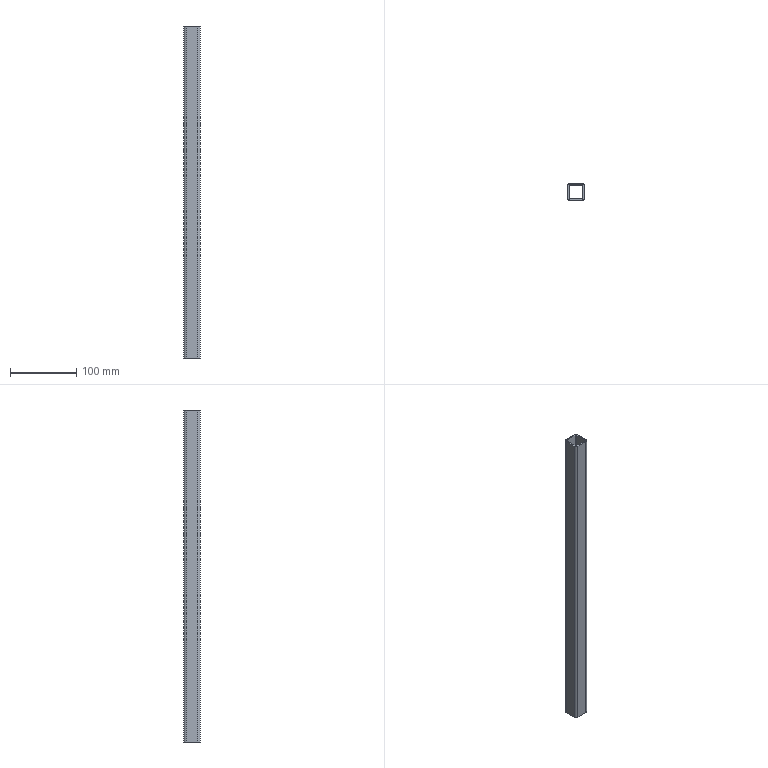Part | SolidWorks | features Extrusion 1 | 1 solid | 18 faces | box 25 x 25 x 500 mm | volume 86850 mm3 | plane 10 | cylinder 8 | commonest cylinder face diameters 4 x4 8 x4
STEP:
#1=CARTESIAN_POINT('',(0.,4.,500.));
#2=VERTEX_POINT('',#1);
#3=CARTESIAN_POINT('',(4.,0.,500.));
#4=VERTEX_POINT('',#3);
#5=CARTESIAN_POINT('',(4.,4.,500.));
#6=DIRECTION('',(0.,0.,1.));
#7=DIRECTION('',(-1.,0.,0.));
#8=AXIS2_PLACEMENT_3D('',#5,#6,#7);
#9=CIRCLE('',#8,4.);
#10=EDGE_CURVE('',#2,#4,#9,.T.);
#11=ORIENTED_EDGE('',*,*,#10,.T.);
#12=CARTESIAN_POINT('',(21.,0.,500.));
#13=VERTEX_POINT('',#12);
#14=CARTESIAN_POINT('',(4.,0.,500.));
#15=DIRECTION('',(1.,0.,0.));
#16=VECTOR('',#15,1000.);
#17=LINE('',#14,#16);
#18=EDGE_CURVE('',#4,#13,#17,.T.);
#19=ORIENTED_EDGE('',*,*,#18,.T.);
#20=CARTESIAN_POINT('',(25.,4.,500.));
#21=VERTEX_POINT('',#20);
#22=CARTESIAN_POINT('',(21.,4.,500.));
#23=DIRECTION('',(0.,0.,1.));
#24=DIRECTION('',(1.,0.,0.));
#25=AXIS2_PLACEMENT_3D('',#22,#23,#24);
#26=CIRCLE('',#25,4.);
#27=EDGE_CURVE('',#13,#21,#26,.T.);
#28=ORIENTED_EDGE('',*,*,#27,.T.);
#29=CARTESIAN_POINT('',(25.,21.,500.));
#30=VERTEX_POINT('',#29);
#31=CARTESIAN_POINT('',(25.,4.,500.));
#32=DIRECTION('',(0.,1.,0.));
#33=VECTOR('',#32,1000.);
#34=LINE('',#31,#33);
#35=EDGE_CURVE('',#21,#30,#34,.T.);
#36=ORIENTED_EDGE('',*,*,#35,.T.);
#37=CARTESIAN_POINT('',(21.,25.,500.));
#38=VERTEX_POINT('',#37);
#39=CARTESIAN_POINT('',(21.,21.,500.));
#40=DIRECTION('',(0.,0.,1.));
#41=DIRECTION('',(-1.,0.,0.));
#42=AXIS2_PLACEMENT_3D('',#39,#40,#41);
#43=CIRCLE('',#42,4.);
#44=EDGE_CURVE('',#30,#38,#43,.T.);
#45=ORIENTED_EDGE('',*,*,#44,.T.);
#46=CARTESIAN_POINT('',(4.,25.,500.));
#47=VERTEX_POINT('',#46);
#48=CARTESIAN_POINT('',(4.,25.,500.));
#49=DIRECTION('',(-1.,0.,0.));
#50=VECTOR('',#49,1000.);
#51=LINE('',#48,#50);
#52=EDGE_CURVE('',#38,#47,#51,.T.);
#53=ORIENTED_EDGE('',*,*,#52,.T.);
#54=CARTESIAN_POINT('',(0.,21.,500.));
#55=VERTEX_POINT('',#54);
#56=CARTESIAN_POINT('',(4.,21.,500.));
#57=DIRECTION('',(0.,0.,1.));
#58=DIRECTION('',(-1.,0.,0.));
#59=AXIS2_PLACEMENT_3D('',#56,#57,#58);
#60=CIRCLE('',#59,4.);
#61=EDGE_CURVE('',#47,#55,#60,.T.);
#62=ORIENTED_EDGE('',*,*,#61,.T.);
#63=CARTESIAN_POINT('',(0.,4.,500.));
#64=DIRECTION('',(0.,-1.,0.));
#65=VECTOR('',#64,1000.);
#66=LINE('',#63,#65);
#67=EDGE_CURVE('',#55,#2,#66,.T.);
#68=ORIENTED_EDGE('',*,*,#67,.T.);
#69=EDGE_LOOP('',(#11,#19,#28,#36,#45,#53,#62,#68));
#70=FACE_OUTER_BOUND('',#69,.T.);
#71=CARTESIAN_POINT('',(23.,21.,500.));
#72=VERTEX_POINT('',#71);
#73=CARTESIAN_POINT('',(21.,23.,500.));
#74=VERTEX_POINT('',#73);
#75=CARTESIAN_POINT('',(21.,21.,500.));
#76=DIRECTION('',(0.,0.,1.));
#77=DIRECTION('',(-1.,0.,0.));
#78=AXIS2_PLACEMENT_3D('',#75,#76,#77);
#79=CIRCLE('',#78,2.);
#80=EDGE_CURVE('',#72,#74,#79,.T.);
#81=ORIENTED_EDGE('',*,*,#80,.F.);
#82=CARTESIAN_POINT('',(23.,4.,500.));
#83=VERTEX_POINT('',#82);
#84=CARTESIAN_POINT('',(23.,4.,500.));
#85=DIRECTION('',(0.,1.,0.));
#86=VECTOR('',#85,1000.);
#87=LINE('',#84,#86);
#88=EDGE_CURVE('',#83,#72,#87,.T.);
#89=ORIENTED_EDGE('',*,*,#88,.F.);
#90=CARTESIAN_POINT('',(21.,2.,500.));
#91=VERTEX_POINT('',#90);
#92=CARTESIAN_POINT('',(21.,4.,500.));
#93=DIRECTION('',(0.,0.,1.));
#94=DIRECTION('',(1.,0.,0.));
#95=AXIS2_PLACEMENT_3D('',#92,#93,#94);
#96=CIRCLE('',#95,2.);
#97=EDGE_CURVE('',#91,#83,#96,.T.);
#98=ORIENTED_EDGE('',*,*,#97,.F.);
#99=CARTESIAN_POINT('',(4.,2.,500.));
#100=VERTEX_POINT('',#99);
#101=CARTESIAN_POINT('',(4.,2.,500.));
#102=DIRECTION('',(1.,0.,0.));
#103=VECTOR('',#102,1000.);
#104=LINE('',#101,#103);
#105=EDGE_CURVE('',#100,#91,#104,.T.);
#106=ORIENTED_EDGE('',*,*,#105,.F.);
#107=CARTESIAN_POINT('',(2.,4.,500.));
#108=VERTEX_POINT('',#107);
#109=CARTESIAN_POINT('',(4.,4.,500.));
#110=DIRECTION('',(0.,0.,1.));
#111=DIRECTION('',(-1.,0.,0.));
#112=AXIS2_PLACEMENT_3D('',#109,#110,#111);
#113=CIRCLE('',#112,2.);
#114=EDGE_CURVE('',#108,#100,#113,.T.);
#115=ORIENTED_EDGE('',*,*,#114,.F.);
#116=CARTESIAN_POINT('',(2.,21.,500.));
#117=VERTEX_POINT('',#116);
#118=CARTESIAN_POINT('',(2.,4.,500.));
#119=DIRECTION('',(0.,-1.,0.));
#120=VECTOR('',#119,1000.);
#121=LINE('',#118,#120);
#122=EDGE_CURVE('',#117,#108,#121,.T.);
#123=ORIENTED_EDGE('',*,*,#122,.F.);
#124=CARTESIAN_POINT('',(4.,23.,500.));
#125=VERTEX_POINT('',#124);
#126=CARTESIAN_POINT('',(4.,21.,500.));
#127=DIRECTION('',(0.,0.,1.));
#128=DIRECTION('',(-1.,0.,0.));
#129=AXIS2_PLACEMENT_3D('',#126,#127,#128);
#130=CIRCLE('',#129,2.);
#131=EDGE_CURVE('',#125,#117,#130,.T.);
#132=ORIENTED_EDGE('',*,*,#131,.F.);
#133=CARTESIAN_POINT('',(4.,23.,500.));
#134=DIRECTION('',(-1.,0.,0.));
#135=VECTOR('',#134,1000.);
#136=LINE('',#133,#135);
#137=EDGE_CURVE('',#74,#125,#136,.T.);
#138=ORIENTED_EDGE('',*,*,#137,.F.);
#139=EDGE_LOOP('',(#81,#89,#98,#106,#115,#123,#132,#138));
#140=FACE_BOUND('',#139,.T.);
#141=CARTESIAN_POINT('',(4.,4.,500.));
#142=DIRECTION('',(0.,0.,-1.));
#143=DIRECTION('',(-1.,0.,0.));
#144=AXIS2_PLACEMENT_3D('',#141,#142,#143);
#145=PLANE('',#144);
#146=ADVANCED_FACE('',(#70,#140),#145,.F.);
#147=CARTESIAN_POINT('',(0.,4.,0.));
#148=VERTEX_POINT('',#147);
#149=CARTESIAN_POINT('',(4.,0.,0.));
#150=VERTEX_POINT('',#149);
#151=CARTESIAN_POINT('',(4.,4.,0.));
#152=DIRECTION('',(0.,0.,1.));
#153=DIRECTION('',(-1.,0.,0.));
#154=AXIS2_PLACEMENT_3D('',#151,#152,#153);
#155=CIRCLE('',#154,4.);
#156=EDGE_CURVE('',#148,#150,#155,.T.);
#157=ORIENTED_EDGE('',*,*,#156,.F.);
#158=CARTESIAN_POINT('',(0.,21.,0.));
#159=VERTEX_POINT('',#158);
#160=CARTESIAN_POINT('',(0.,4.,0.));
#161=DIRECTION('',(0.,-1.,0.));
#162=VECTOR('',#161,1000.);
#163=LINE('',#160,#162);
#164=EDGE_CURVE('',#159,#148,#163,.T.);
#165=ORIENTED_EDGE('',*,*,#164,.F.);
#166=CARTESIAN_POINT('',(4.,25.,0.));
#167=VERTEX_POINT('',#166);
#168=CARTESIAN_POINT('',(4.,21.,0.));
#169=DIRECTION('',(0.,0.,1.));
#170=DIRECTION('',(-1.,0.,0.));
#171=AXIS2_PLACEMENT_3D('',#168,#169,#170);
#172=CIRCLE('',#171,4.);
#173=EDGE_CURVE('',#167,#159,#172,.T.);
#174=ORIENTED_EDGE('',*,*,#173,.F.);
#175=CARTESIAN_POINT('',(21.,25.,0.));
#176=VERTEX_POINT('',#175);
#177=CARTESIAN_POINT('',(4.,25.,0.));
#178=DIRECTION('',(-1.,0.,0.));
#179=VECTOR('',#178,1000.);
#180=LINE('',#177,#179);
#181=EDGE_CURVE('',#176,#167,#180,.T.);
#182=ORIENTED_EDGE('',*,*,#181,.F.);
#183=CARTESIAN_POINT('',(25.,21.,0.));
#184=VERTEX_POINT('',#183);
#185=CARTESIAN_POINT('',(21.,21.,0.));
#186=DIRECTION('',(0.,0.,1.));
#187=DIRECTION('',(-1.,0.,0.));
#188=AXIS2_PLACEMENT_3D('',#185,#186,#187);
#189=CIRCLE('',#188,4.);
#190=EDGE_CURVE('',#184,#176,#189,.T.);
#191=ORIENTED_EDGE('',*,*,#190,.F.);
#192=CARTESIAN_POINT('',(25.,4.,0.));
#193=VERTEX_POINT('',#192);
#194=CARTESIAN_POINT('',(25.,4.,0.));
#195=DIRECTION('',(0.,1.,0.));
#196=VECTOR('',#195,1000.);
#197=LINE('',#194,#196);
#198=EDGE_CURVE('',#193,#184,#197,.T.);
#199=ORIENTED_EDGE('',*,*,#198,.F.);
#200=CARTESIAN_POINT('',(21.,0.,0.));
#201=VERTEX_POINT('',#200);
#202=CARTESIAN_POINT('',(21.,4.,0.));
#203=DIRECTION('',(0.,0.,1.));
#204=DIRECTION('',(1.,0.,0.));
#205=AXIS2_PLACEMENT_3D('',#202,#203,#204);
#206=CIRCLE('',#205,4.);
#207=EDGE_CURVE('',#201,#193,#206,.T.);
#208=ORIENTED_EDGE('',*,*,#207,.F.);
#209=CARTESIAN_POINT('',(4.,0.,0.));
#210=DIRECTION('',(1.,0.,0.));
#211=VECTOR('',#210,1000.);
#212=LINE('',#209,#211);
#213=EDGE_CURVE('',#150,#201,#212,.T.);
#214=ORIENTED_EDGE('',*,*,#213,.F.);
#215=EDGE_LOOP('',(#157,#165,#174,#182,#191,#199,#208,#214));
#216=FACE_OUTER_BOUND('',#215,.T.);
#217=CARTESIAN_POINT('',(23.,4.,0.));
#218=VERTEX_POINT('',#217);
#219=CARTESIAN_POINT('',(23.,21.,0.));
#220=VERTEX_POINT('',#219);
#221=CARTESIAN_POINT('',(23.,4.,0.));
#222=DIRECTION('',(0.,1.,0.));
#223=VECTOR('',#222,1000.);
#224=LINE('',#221,#223);
#225=EDGE_CURVE('',#218,#220,#224,.T.);
#226=ORIENTED_EDGE('',*,*,#225,.T.);
#227=CARTESIAN_POINT('',(21.,23.,0.));
#228=VERTEX_POINT('',#227);
#229=CARTESIAN_POINT('',(21.,21.,0.));
#230=DIRECTION('',(0.,0.,1.));
#231=DIRECTION('',(-1.,0.,0.));
#232=AXIS2_PLACEMENT_3D('',#229,#230,#231);
#233=CIRCLE('',#232,2.);
#234=EDGE_CURVE('',#220,#228,#233,.T.);
#235=ORIENTED_EDGE('',*,*,#234,.T.);
#236=CARTESIAN_POINT('',(4.,23.,0.));
#237=VERTEX_POINT('',#236);
#238=CARTESIAN_POINT('',(4.,23.,0.));
#239=DIRECTION('',(-1.,0.,0.));
#240=VECTOR('',#239,1000.);
#241=LINE('',#238,#240);
#242=EDGE_CURVE('',#228,#237,#241,.T.);
#243=ORIENTED_EDGE('',*,*,#242,.T.);
#244=CARTESIAN_POINT('',(2.,21.,0.));
#245=VERTEX_POINT('',#244);
#246=CARTESIAN_POINT('',(4.,21.,0.));
#247=DIRECTION('',(0.,0.,1.));
#248=DIRECTION('',(-1.,0.,0.));
#249=AXIS2_PLACEMENT_3D('',#246,#247,#248);
#250=CIRCLE('',#249,2.);
#251=EDGE_CURVE('',#237,#245,#250,.T.);
#252=ORIENTED_EDGE('',*,*,#251,.T.);
#253=CARTESIAN_POINT('',(2.,4.,0.));
#254=VERTEX_POINT('',#253);
#255=CARTESIAN_POINT('',(2.,4.,0.));
#256=DIRECTION('',(0.,-1.,0.));
#257=VECTOR('',#256,1000.);
#258=LINE('',#255,#257);
#259=EDGE_CURVE('',#245,#254,#258,.T.);
#260=ORIENTED_EDGE('',*,*,#259,.T.);
#261=CARTESIAN_POINT('',(4.,2.,0.));
#262=VERTEX_POINT('',#261);
#263=CARTESIAN_POINT('',(4.,4.,0.));
#264=DIRECTION('',(0.,0.,1.));
#265=DIRECTION('',(-1.,0.,0.));
#266=AXIS2_PLACEMENT_3D('',#263,#264,#265);
#267=CIRCLE('',#266,2.);
#268=EDGE_CURVE('',#254,#262,#267,.T.);
#269=ORIENTED_EDGE('',*,*,#268,.T.);
#270=CARTESIAN_POINT('',(21.,2.,0.));
#271=VERTEX_POINT('',#270);
#272=CARTESIAN_POINT('',(4.,2.,0.));
#273=DIRECTION('',(1.,0.,0.));
#274=VECTOR('',#273,1000.);
#275=LINE('',#272,#274);
#276=EDGE_CURVE('',#262,#271,#275,.T.);
#277=ORIENTED_EDGE('',*,*,#276,.T.);
#278=CARTESIAN_POINT('',(21.,4.,0.));
#279=DIRECTION('',(0.,0.,1.));
#280=DIRECTION('',(1.,0.,0.));
#281=AXIS2_PLACEMENT_3D('',#278,#279,#280);
#282=CIRCLE('',#281,2.);
#283=EDGE_CURVE('',#271,#218,#282,.T.);
#284=ORIENTED_EDGE('',*,*,#283,.T.);
#285=EDGE_LOOP('',(#226,#235,#243,#252,#260,#269,#277,#284));
#286=FACE_BOUND('',#285,.T.);
#287=CARTESIAN_POINT('',(4.,4.,0.));
#288=DIRECTION('',(0.,0.,-1.));
#289=DIRECTION('',(-1.,0.,0.));
#290=AXIS2_PLACEMENT_3D('',#287,#288,#289);
#291=PLANE('',#290);
#292=ADVANCED_FACE('',(#216,#286),#291,.T.);
#293=ORIENTED_EDGE('',*,*,#156,.T.);
#294=CARTESIAN_POINT('',(4.,0.,500.));
#295=DIRECTION('',(0.,0.,-1.));
#296=VECTOR('',#295,1000.);
#297=LINE('',#294,#296);
#298=EDGE_CURVE('',#4,#150,#297,.T.);
#299=ORIENTED_EDGE('',*,*,#298,.F.);
#300=ORIENTED_EDGE('',*,*,#10,.F.);
#301=CARTESIAN_POINT('',(0.,4.,500.));
#302=DIRECTION('',(0.,0.,-1.));
#303=VECTOR('',#302,1000.);
#304=LINE('',#301,#303);
#305=EDGE_CURVE('',#2,#148,#304,.T.);
#306=ORIENTED_EDGE('',*,*,#305,.T.);
#307=EDGE_LOOP('',(#293,#299,#300,#306));
#308=FACE_OUTER_BOUND('',#307,.T.);
#309=CARTESIAN_POINT('',(4.,4.,500.));
#310=DIRECTION('',(0.,0.,-1.));
#311=DIRECTION('',(-1.,0.,0.));
#312=AXIS2_PLACEMENT_3D('',#309,#310,#311);
#313=CYLINDRICAL_SURFACE('',#312,4.);
#314=ADVANCED_FACE('',(#308),#313,.T.);
#315=ORIENTED_EDGE('',*,*,#213,.T.);
#316=CARTESIAN_POINT('',(21.,0.,500.));
#317=DIRECTION('',(0.,0.,-1.));
#318=VECTOR('',#317,1000.);
#319=LINE('',#316,#318);
#320=EDGE_CURVE('',#13,#201,#319,.T.);
#321=ORIENTED_EDGE('',*,*,#320,.F.);
#322=ORIENTED_EDGE('',*,*,#18,.F.);
#323=ORIENTED_EDGE('',*,*,#298,.T.);
#324=EDGE_LOOP('',(#315,#321,#322,#323));
#325=FACE_OUTER_BOUND('',#324,.T.);
#326=CARTESIAN_POINT('',(4.,0.,500.));
#327=DIRECTION('',(0.,1.,0.));
#328=DIRECTION('',(0.,0.,1.));
#329=AXIS2_PLACEMENT_3D('',#326,#327,#328);
#330=PLANE('',#329);
#331=ADVANCED_FACE('',(#325),#330,.F.);
#332=ORIENTED_EDGE('',*,*,#207,.T.);
#333=CARTESIAN_POINT('',(25.,4.,500.));
#334=DIRECTION('',(0.,0.,-1.));
#335=VECTOR('',#334,1000.);
#336=LINE('',#333,#335);
#337=EDGE_CURVE('',#21,#193,#336,.T.);
#338=ORIENTED_EDGE('',*,*,#337,.F.);
#339=ORIENTED_EDGE('',*,*,#27,.F.);
#340=ORIENTED_EDGE('',*,*,#320,.T.);
#341=EDGE_LOOP('',(#332,#338,#339,#340));
#342=FACE_OUTER_BOUND('',#341,.T.);
#343=CARTESIAN_POINT('',(21.,4.,500.));
#344=DIRECTION('',(0.,0.,-1.));
#345=DIRECTION('',(-1.,0.,0.));
#346=AXIS2_PLACEMENT_3D('',#343,#344,#345);
#347=CYLINDRICAL_SURFACE('',#346,4.);
#348=ADVANCED_FACE('',(#342),#347,.T.);
#349=ORIENTED_EDGE('',*,*,#198,.T.);
#350=CARTESIAN_POINT('',(25.,21.,500.));
#351=DIRECTION('',(0.,0.,-1.));
#352=VECTOR('',#351,1000.);
#353=LINE('',#350,#352);
#354=EDGE_CURVE('',#30,#184,#353,.T.);
#355=ORIENTED_EDGE('',*,*,#354,.F.);
#356=ORIENTED_EDGE('',*,*,#35,.F.);
#357=ORIENTED_EDGE('',*,*,#337,.T.);
#358=EDGE_LOOP('',(#349,#355,#356,#357));
#359=FACE_OUTER_BOUND('',#358,.T.);
#360=CARTESIAN_POINT('',(25.,4.,500.));
#361=DIRECTION('',(-1.,0.,0.));
#362=DIRECTION('',(0.,0.,1.));
#363=AXIS2_PLACEMENT_3D('',#360,#361,#362);
#364=PLANE('',#363);
#365=ADVANCED_FACE('',(#359),#364,.F.);
#366=ORIENTED_EDGE('',*,*,#190,.T.);
#367=CARTESIAN_POINT('',(21.,25.,500.));
#368=DIRECTION('',(0.,0.,-1.));
#369=VECTOR('',#368,1000.);
#370=LINE('',#367,#369);
#371=EDGE_CURVE('',#38,#176,#370,.T.);
#372=ORIENTED_EDGE('',*,*,#371,.F.);
#373=ORIENTED_EDGE('',*,*,#44,.F.);
#374=ORIENTED_EDGE('',*,*,#354,.T.);
#375=EDGE_LOOP('',(#366,#372,#373,#374));
#376=FACE_OUTER_BOUND('',#375,.T.);
#377=CARTESIAN_POINT('',(21.,21.,500.));
#378=DIRECTION('',(0.,0.,-1.));
#379=DIRECTION('',(-1.,0.,0.));
#380=AXIS2_PLACEMENT_3D('',#377,#378,#379);
#381=CYLINDRICAL_SURFACE('',#380,4.);
#382=ADVANCED_FACE('',(#376),#381,.T.);
#383=ORIENTED_EDGE('',*,*,#181,.T.);
#384=CARTESIAN_POINT('',(4.,25.,500.));
#385=DIRECTION('',(0.,0.,-1.));
#386=VECTOR('',#385,1000.);
#387=LINE('',#384,#386);
#388=EDGE_CURVE('',#47,#167,#387,.T.);
#389=ORIENTED_EDGE('',*,*,#388,.F.);
#390=ORIENTED_EDGE('',*,*,#52,.F.);
#391=ORIENTED_EDGE('',*,*,#371,.T.);
#392=EDGE_LOOP('',(#383,#389,#390,#391));
#393=FACE_OUTER_BOUND('',#392,.T.);
#394=CARTESIAN_POINT('',(4.,25.,500.));
#395=DIRECTION('',(0.,-1.,0.));
#396=DIRECTION('',(0.,0.,-1.));
#397=AXIS2_PLACEMENT_3D('',#394,#395,#396);
#398=PLANE('',#397);
#399=ADVANCED_FACE('',(#393),#398,.F.);
#400=ORIENTED_EDGE('',*,*,#173,.T.);
#401=CARTESIAN_POINT('',(0.,21.,500.));
#402=DIRECTION('',(0.,0.,-1.));
#403=VECTOR('',#402,1000.);
#404=LINE('',#401,#403);
#405=EDGE_CURVE('',#55,#159,#404,.T.);
#406=ORIENTED_EDGE('',*,*,#405,.F.);
#407=ORIENTED_EDGE('',*,*,#61,.F.);
#408=ORIENTED_EDGE('',*,*,#388,.T.);
#409=EDGE_LOOP('',(#400,#406,#407,#408));
#410=FACE_OUTER_BOUND('',#409,.T.);
#411=CARTESIAN_POINT('',(4.,21.,500.));
#412=DIRECTION('',(0.,0.,-1.));
#413=DIRECTION('',(-1.,0.,0.));
#414=AXIS2_PLACEMENT_3D('',#411,#412,#413);
#415=CYLINDRICAL_SURFACE('',#414,4.);
#416=ADVANCED_FACE('',(#410),#415,.T.);
#417=ORIENTED_EDGE('',*,*,#164,.T.);
#418=ORIENTED_EDGE('',*,*,#305,.F.);
#419=ORIENTED_EDGE('',*,*,#67,.F.);
#420=ORIENTED_EDGE('',*,*,#405,.T.);
#421=EDGE_LOOP('',(#417,#418,#419,#420));
#422=FACE_OUTER_BOUND('',#421,.T.);
#423=CARTESIAN_POINT('',(0.,4.,500.));
#424=DIRECTION('',(1.,0.,0.));
#425=DIRECTION('',(0.,0.,-1.));
#426=AXIS2_PLACEMENT_3D('',#423,#424,#425);
#427=PLANE('',#426);
#428=ADVANCED_FACE('',(#422),#427,.F.);
#429=ORIENTED_EDGE('',*,*,#234,.F.);
#430=CARTESIAN_POINT('',(23.,21.,500.));
#431=DIRECTION('',(0.,0.,-1.));
#432=VECTOR('',#431,1000.);
#433=LINE('',#430,#432);
#434=EDGE_CURVE('',#72,#220,#433,.T.);
#435=ORIENTED_EDGE('',*,*,#434,.F.);
#436=ORIENTED_EDGE('',*,*,#80,.T.);
#437=CARTESIAN_POINT('',(21.,23.,500.));
#438=DIRECTION('',(0.,0.,-1.));
#439=VECTOR('',#438,1000.);
#440=LINE('',#437,#439);
#441=EDGE_CURVE('',#74,#228,#440,.T.);
#442=ORIENTED_EDGE('',*,*,#441,.T.);
#443=EDGE_LOOP('',(#429,#435,#436,#442));
#444=FACE_OUTER_BOUND('',#443,.T.);
#445=CARTESIAN_POINT('',(21.,21.,500.));
#446=DIRECTION('',(0.,0.,-1.));
#447=DIRECTION('',(-1.,0.,0.));
#448=AXIS2_PLACEMENT_3D('',#445,#446,#447);
#449=CYLINDRICAL_SURFACE('',#448,2.);
#450=ADVANCED_FACE('',(#444),#449,.F.);
#451=ORIENTED_EDGE('',*,*,#242,.F.);
#452=ORIENTED_EDGE('',*,*,#441,.F.);
#453=ORIENTED_EDGE('',*,*,#137,.T.);
#454=CARTESIAN_POINT('',(4.,23.,500.));
#455=DIRECTION('',(0.,0.,-1.));
#456=VECTOR('',#455,1000.);
#457=LINE('',#454,#456);
#458=EDGE_CURVE('',#125,#237,#457,.T.);
#459=ORIENTED_EDGE('',*,*,#458,.T.);
#460=EDGE_LOOP('',(#451,#452,#453,#459));
#461=FACE_OUTER_BOUND('',#460,.T.);
#462=CARTESIAN_POINT('',(4.,23.,500.));
#463=DIRECTION('',(0.,-1.,0.));
#464=DIRECTION('',(0.,0.,-1.));
#465=AXIS2_PLACEMENT_3D('',#462,#463,#464);
#466=PLANE('',#465);
#467=ADVANCED_FACE('',(#461),#466,.T.);
#468=ORIENTED_EDGE('',*,*,#251,.F.);
#469=ORIENTED_EDGE('',*,*,#458,.F.);
#470=ORIENTED_EDGE('',*,*,#131,.T.);
#471=CARTESIAN_POINT('',(2.,21.,500.));
#472=DIRECTION('',(0.,0.,-1.));
#473=VECTOR('',#472,1000.);
#474=LINE('',#471,#473);
#475=EDGE_CURVE('',#117,#245,#474,.T.);
#476=ORIENTED_EDGE('',*,*,#475,.T.);
#477=EDGE_LOOP('',(#468,#469,#470,#476));
#478=FACE_OUTER_BOUND('',#477,.T.);
#479=CARTESIAN_POINT('',(4.,21.,500.));
#480=DIRECTION('',(0.,0.,-1.));
#481=DIRECTION('',(-1.,0.,0.));
#482=AXIS2_PLACEMENT_3D('',#479,#480,#481);
#483=CYLINDRICAL_SURFACE('',#482,2.);
#484=ADVANCED_FACE('',(#478),#483,.F.);
#485=ORIENTED_EDGE('',*,*,#259,.F.);
#486=ORIENTED_EDGE('',*,*,#475,.F.);
#487=ORIENTED_EDGE('',*,*,#122,.T.);
#488=CARTESIAN_POINT('',(2.,4.,500.));
#489=DIRECTION('',(0.,0.,-1.));
#490=VECTOR('',#489,1000.);
#491=LINE('',#488,#490);
#492=EDGE_CURVE('',#108,#254,#491,.T.);
#493=ORIENTED_EDGE('',*,*,#492,.T.);
#494=EDGE_LOOP('',(#485,#486,#487,#493));
#495=FACE_OUTER_BOUND('',#494,.T.);
#496=CARTESIAN_POINT('',(2.,4.,500.));
#497=DIRECTION('',(1.,0.,0.));
#498=DIRECTION('',(0.,0.,-1.));
#499=AXIS2_PLACEMENT_3D('',#496,#497,#498);
#500=PLANE('',#499);
#501=ADVANCED_FACE('',(#495),#500,.T.);
#502=ORIENTED_EDGE('',*,*,#268,.F.);
#503=ORIENTED_EDGE('',*,*,#492,.F.);
#504=ORIENTED_EDGE('',*,*,#114,.T.);
#505=CARTESIAN_POINT('',(4.,2.,500.));
#506=DIRECTION('',(0.,0.,-1.));
#507=VECTOR('',#506,1000.);
#508=LINE('',#505,#507);
#509=EDGE_CURVE('',#100,#262,#508,.T.);
#510=ORIENTED_EDGE('',*,*,#509,.T.);
#511=EDGE_LOOP('',(#502,#503,#504,#510));
#512=FACE_OUTER_BOUND('',#511,.T.);
#513=CARTESIAN_POINT('',(4.,4.,500.));
#514=DIRECTION('',(0.,0.,-1.));
#515=DIRECTION('',(-1.,0.,0.));
#516=AXIS2_PLACEMENT_3D('',#513,#514,#515);
#517=CYLINDRICAL_SURFACE('',#516,2.);
#518=ADVANCED_FACE('',(#512),#517,.F.);
#519=ORIENTED_EDGE('',*,*,#276,.F.);
#520=ORIENTED_EDGE('',*,*,#509,.F.);
#521=ORIENTED_EDGE('',*,*,#105,.T.);
#522=CARTESIAN_POINT('',(21.,2.,500.));
#523=DIRECTION('',(0.,0.,-1.));
#524=VECTOR('',#523,1000.);
#525=LINE('',#522,#524);
#526=EDGE_CURVE('',#91,#271,#525,.T.);
#527=ORIENTED_EDGE('',*,*,#526,.T.);
#528=EDGE_LOOP('',(#519,#520,#521,#527));
#529=FACE_OUTER_BOUND('',#528,.T.);
#530=CARTESIAN_POINT('',(4.,2.,500.));
#531=DIRECTION('',(0.,1.,0.));
#532=DIRECTION('',(0.,0.,1.));
#533=AXIS2_PLACEMENT_3D('',#530,#531,#532);
#534=PLANE('',#533);
#535=ADVANCED_FACE('',(#529),#534,.T.);
#536=ORIENTED_EDGE('',*,*,#283,.F.);
#537=ORIENTED_EDGE('',*,*,#526,.F.);
#538=ORIENTED_EDGE('',*,*,#97,.T.);
#539=CARTESIAN_POINT('',(23.,4.,500.));
#540=DIRECTION('',(0.,0.,-1.));
#541=VECTOR('',#540,1000.);
#542=LINE('',#539,#541);
#543=EDGE_CURVE('',#83,#218,#542,.T.);
#544=ORIENTED_EDGE('',*,*,#543,.T.);
#545=EDGE_LOOP('',(#536,#537,#538,#544));
#546=FACE_OUTER_BOUND('',#545,.T.);
#547=CARTESIAN_POINT('',(21.,4.,500.));
#548=DIRECTION('',(0.,0.,-1.));
#549=DIRECTION('',(-1.,0.,0.));
#550=AXIS2_PLACEMENT_3D('',#547,#548,#549);
#551=CYLINDRICAL_SURFACE('',#550,2.);
#552=ADVANCED_FACE('',(#546),#551,.F.);
#553=ORIENTED_EDGE('',*,*,#225,.F.);
#554=ORIENTED_EDGE('',*,*,#543,.F.);
#555=ORIENTED_EDGE('',*,*,#88,.T.);
#556=ORIENTED_EDGE('',*,*,#434,.T.);
#557=EDGE_LOOP('',(#553,#554,#555,#556));
#558=FACE_OUTER_BOUND('',#557,.T.);
#559=CARTESIAN_POINT('',(23.,4.,500.));
#560=DIRECTION('',(-1.,0.,0.));
#561=DIRECTION('',(0.,0.,1.));
#562=AXIS2_PLACEMENT_3D('',#559,#560,#561);
#563=PLANE('',#562);
#564=ADVANCED_FACE('',(#558),#563,.T.);
#565=CLOSED_SHELL('',(#146,#292,#314,#331,#348,#365,#382,#399,#416,#428,#450,#467,#484,#501,#518,#535,#552,#564));
#566=MANIFOLD_SOLID_BREP('',#565);
#567=CARTESIAN_POINT('',(0.,0.,0.));
#568=DIRECTION('',(0.,0.,1.));
#569=DIRECTION('',(1.,0.,0.));
#570=AXIS2_PLACEMENT_3D('',#567,#568,#569);
#571=(LENGTH_UNIT()NAMED_UNIT(*)SI_UNIT(.MILLI.,.METRE.));
#572=UNCERTAINTY_MEASURE_WITH_UNIT(LENGTH_MEASURE(0.00001),#571,'','');
#573=(NAMED_UNIT(*)PLANE_ANGLE_UNIT()SI_UNIT($,.RADIAN.));
#574=(NAMED_UNIT(*)SI_UNIT($,.STERADIAN.)SOLID_ANGLE_UNIT());
#575=(GEOMETRIC_REPRESENTATION_CONTEXT(3)GLOBAL_UNCERTAINTY_ASSIGNED_CONTEXT((#572))GLOBAL_UNIT_ASSIGNED_CONTEXT((#571,#573,#574))REPRESENTATION_CONTEXT('',''));
#576=ADVANCED_BREP_SHAPE_REPRESENTATION('',(#566,#570),#575);